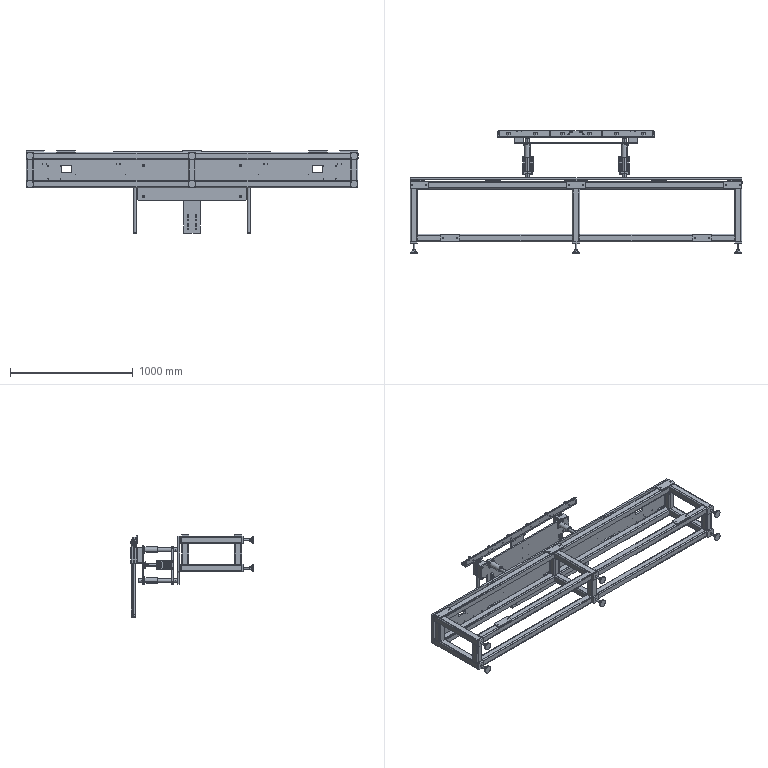Part | SolidWorks | features ReferencePattern 11, DerivedHolePattern 2, CompositeCurve 1 | 107 solids | 3854 faces | volume 41125199 mm3 | cylinder 1752 | plane 1400 | cone 574 | spline 128 | commonest cylinder face diameters 6.8 x140 11 x124 6.6 x108 10 x108 5 x104 3.3 x88